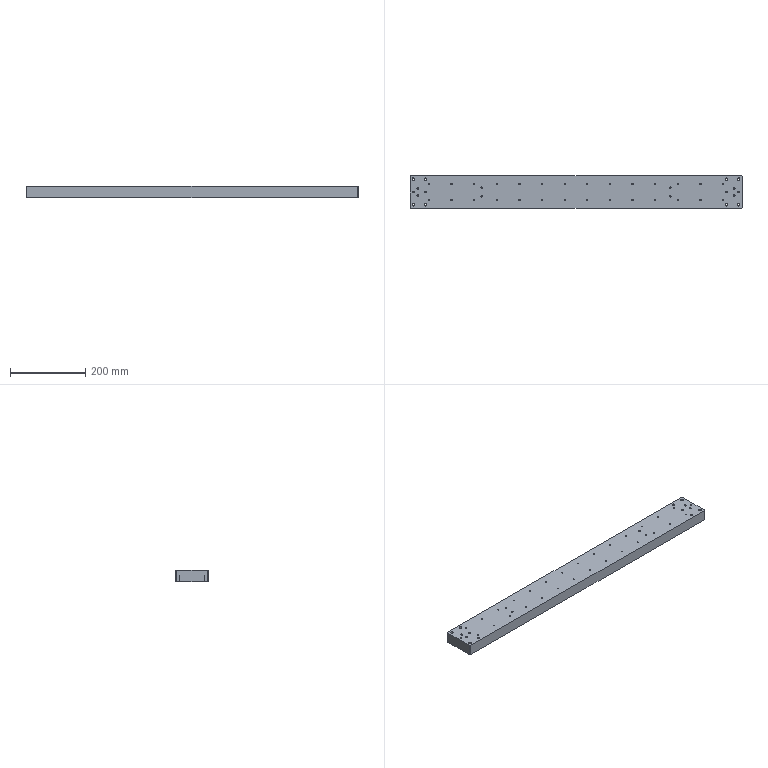Part | STEP file | 1 solid | 154 faces | box 880 x 86 x 30 mm | volume 2237811 mm3 | cylinder 128 | plane 26 | commonest cylinder face diameters 3.3 x56 5 x24 6.6 x16 11 x16 4 x8 8 x8